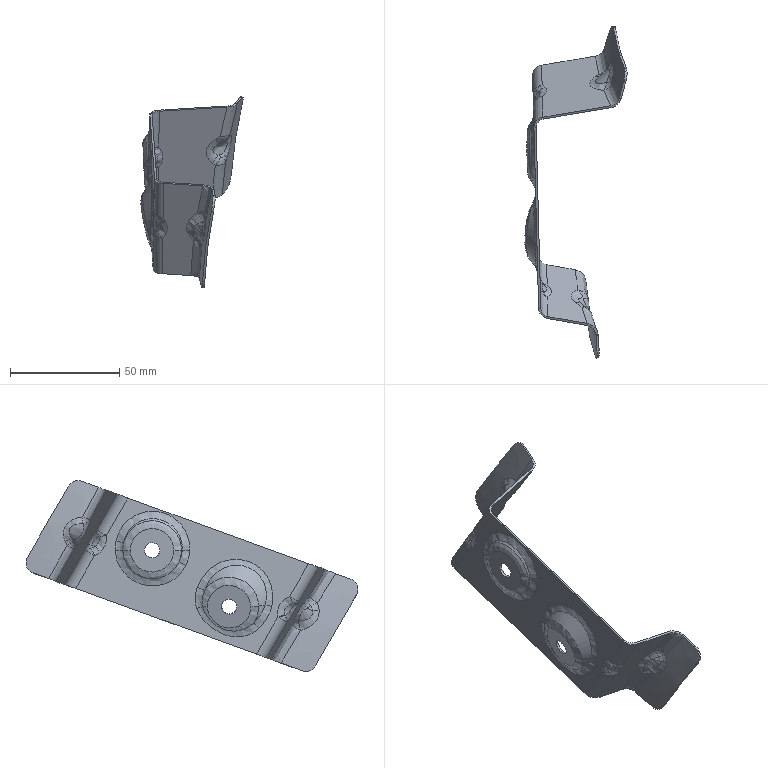Part | 1 solid | 154 faces | box 46.756 x 151.876 x 87.338 mm | volume 8763 mm3 | spline 118 | sphere 16 | cylinder 12 | plane 8 | commonest cylinder face diameters 7 x4 8 x4 10 x4